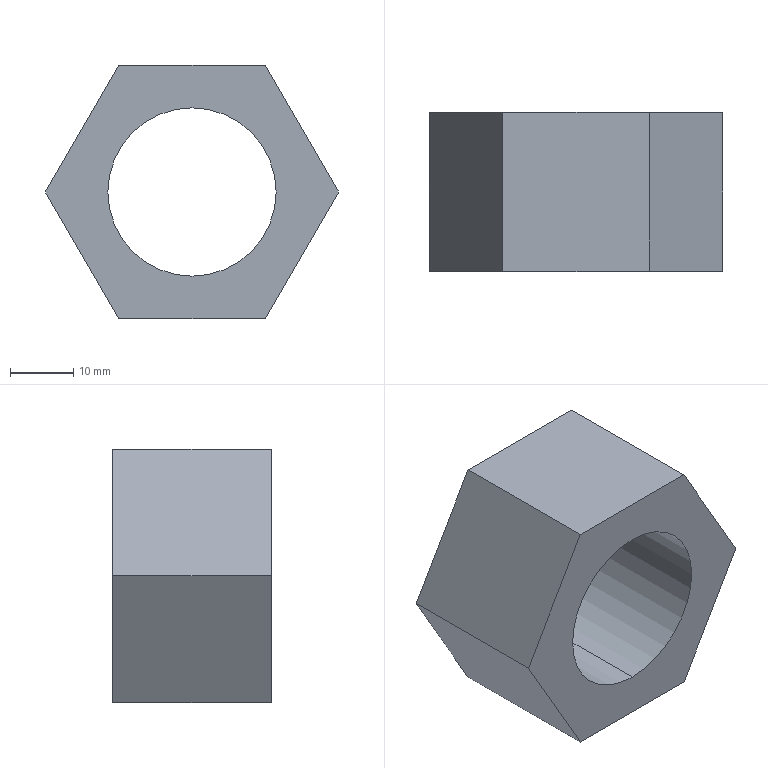Part | STEP file | 1 solid | 10 faces | box 46.188 x 25 x 40 mm | volume 20852 mm3 | plane 8 | cylinder 2 | commonest cylinder face diameters 26.5 x2
STEP:
#1=CARTESIAN_POINT('',(0.,0.,0.));
#2=DIRECTION('',(0.,0.,1.));
#3=DIRECTION('',(1.,0.,0.));
#4=AXIS2_PLACEMENT_3D('',#1,#2,#3);
#5=CARTESIAN_POINT('',(0.,0.,13.25));
#6=VERTEX_POINT('',#5);
#7=CARTESIAN_POINT('',(0.,25.,13.25));
#8=VERTEX_POINT('',#7);
#9=CARTESIAN_POINT('',(0.,0.,13.25));
#10=DIRECTION('',(0.,1.,0.));
#11=VECTOR('',#10,1.);
#12=LINE('',#9,#11);
#13=CARTESIAN_POINT('',(0.,0.,0.));
#14=DIRECTION('',(0.,1.,0.));
#15=DIRECTION('',(0.,0.,1.));
#16=AXIS2_PLACEMENT_3D('',#13,#14,#15);
#17=CYLINDRICAL_SURFACE('',#16,13.25);
#18=CARTESIAN_POINT('',(6.283,0.));
#19=DIRECTION('',(0.,1.));
#20=VECTOR('',#19,1.);
#21=LINE('',#18,#20);
#22=(GEOMETRIC_REPRESENTATION_CONTEXT(2)PARAMETRIC_REPRESENTATION_CONTEXT()REPRESENTATION_CONTEXT('',''));
#23=DEFINITIONAL_REPRESENTATION('',(#21),#22);
#24=PCURVE('',#17,#23);
#25=CARTESIAN_POINT('',(0.,0.,0.));
#26=DIRECTION('',(0.,1.,0.));
#27=DIRECTION('',(0.,0.,1.));
#28=AXIS2_PLACEMENT_3D('',#25,#26,#27);
#29=CYLINDRICAL_SURFACE('',#28,13.25);
#30=CARTESIAN_POINT('',(0.,0.));
#31=DIRECTION('',(0.,1.));
#32=VECTOR('',#31,1.);
#33=LINE('',#30,#32);
#34=(GEOMETRIC_REPRESENTATION_CONTEXT(2)PARAMETRIC_REPRESENTATION_CONTEXT()REPRESENTATION_CONTEXT('',''));
#35=DEFINITIONAL_REPRESENTATION('',(#33),#34);
#36=PCURVE('',#29,#35);
#37=SURFACE_CURVE('',#12,(#24,#36),.PCURVE_S1.);
#38=EDGE_CURVE('',#6,#8,#37,.T.);
#39=ORIENTED_EDGE('',*,*,#38,.T.);
#40=CARTESIAN_POINT('',(0.,25.,-13.25));
#41=VERTEX_POINT('',#40);
#42=CARTESIAN_POINT('',(0.,25.,0.));
#43=DIRECTION('',(0.,1.,0.));
#44=DIRECTION('',(0.,0.,1.));
#45=AXIS2_PLACEMENT_3D('',#42,#43,#44);
#46=CIRCLE('',#45,13.25);
#47=CARTESIAN_POINT('',(0.,25.));
#48=DIRECTION('',(1.,0.));
#49=VECTOR('',#48,1.);
#50=LINE('',#47,#49);
#51=(GEOMETRIC_REPRESENTATION_CONTEXT(2)PARAMETRIC_REPRESENTATION_CONTEXT()REPRESENTATION_CONTEXT('',''));
#52=DEFINITIONAL_REPRESENTATION('',(#50),#51);
#53=PCURVE('',#17,#52);
#54=CARTESIAN_POINT('',(0.,25.,0.));
#55=DIRECTION('',(0.,1.,0.));
#56=DIRECTION('',(0.,0.,1.));
#57=AXIS2_PLACEMENT_3D('',#54,#55,#56);
#58=PLANE('',#57);
#59=CARTESIAN_POINT('',(0.,0.));
#60=DIRECTION('',(1.,0.));
#61=AXIS2_PLACEMENT_2D('',#59,#60);
#62=CIRCLE('',#61,13.25);
#63=(GEOMETRIC_REPRESENTATION_CONTEXT(2)PARAMETRIC_REPRESENTATION_CONTEXT()REPRESENTATION_CONTEXT('',''));
#64=DEFINITIONAL_REPRESENTATION('',(#62),#63);
#65=PCURVE('',#58,#64);
#66=SURFACE_CURVE('',#46,(#53,#65),.PCURVE_S1.);
#67=EDGE_CURVE('',#41,#8,#66,.T.);
#68=ORIENTED_EDGE('',*,*,#67,.F.);
#69=CARTESIAN_POINT('',(0.,0.,-13.25));
#70=VERTEX_POINT('',#69);
#71=CARTESIAN_POINT('',(0.,0.,-13.25));
#72=DIRECTION('',(0.,1.,0.));
#73=VECTOR('',#72,1.);
#74=LINE('',#71,#73);
#75=CARTESIAN_POINT('',(3.142,0.));
#76=DIRECTION('',(0.,1.));
#77=VECTOR('',#76,1.);
#78=LINE('',#75,#77);
#79=(GEOMETRIC_REPRESENTATION_CONTEXT(2)PARAMETRIC_REPRESENTATION_CONTEXT()REPRESENTATION_CONTEXT('',''));
#80=DEFINITIONAL_REPRESENTATION('',(#78),#79);
#81=PCURVE('',#17,#80);
#82=CARTESIAN_POINT('',(3.142,0.));
#83=DIRECTION('',(0.,1.));
#84=VECTOR('',#83,1.);
#85=LINE('',#82,#84);
#86=(GEOMETRIC_REPRESENTATION_CONTEXT(2)PARAMETRIC_REPRESENTATION_CONTEXT()REPRESENTATION_CONTEXT('',''));
#87=DEFINITIONAL_REPRESENTATION('',(#85),#86);
#88=PCURVE('',#29,#87);
#89=SURFACE_CURVE('',#74,(#81,#88),.PCURVE_S1.);
#90=EDGE_CURVE('',#70,#41,#89,.T.);
#91=ORIENTED_EDGE('',*,*,#90,.F.);
#92=CARTESIAN_POINT('',(0.,0.,0.));
#93=DIRECTION('',(0.,1.,0.));
#94=DIRECTION('',(0.,0.,1.));
#95=AXIS2_PLACEMENT_3D('',#92,#93,#94);
#96=CIRCLE('',#95,13.25);
#97=CARTESIAN_POINT('',(0.,0.));
#98=DIRECTION('',(1.,0.));
#99=VECTOR('',#98,1.);
#100=LINE('',#97,#99);
#101=(GEOMETRIC_REPRESENTATION_CONTEXT(2)PARAMETRIC_REPRESENTATION_CONTEXT()REPRESENTATION_CONTEXT('',''));
#102=DEFINITIONAL_REPRESENTATION('',(#100),#101);
#103=PCURVE('',#17,#102);
#104=CARTESIAN_POINT('',(0.,0.,0.));
#105=DIRECTION('',(0.,1.,0.));
#106=DIRECTION('',(0.,0.,1.));
#107=AXIS2_PLACEMENT_3D('',#104,#105,#106);
#108=PLANE('',#107);
#109=CARTESIAN_POINT('',(0.,0.));
#110=DIRECTION('',(1.,0.));
#111=AXIS2_PLACEMENT_2D('',#109,#110);
#112=CIRCLE('',#111,13.25);
#113=(GEOMETRIC_REPRESENTATION_CONTEXT(2)PARAMETRIC_REPRESENTATION_CONTEXT()REPRESENTATION_CONTEXT('',''));
#114=DEFINITIONAL_REPRESENTATION('',(#112),#113);
#115=PCURVE('',#108,#114);
#116=SURFACE_CURVE('',#96,(#103,#115),.PCURVE_S1.);
#117=EDGE_CURVE('',#70,#6,#116,.T.);
#118=ORIENTED_EDGE('',*,*,#117,.T.);
#119=EDGE_LOOP('',(#39,#68,#91,#118));
#120=FACE_BOUND('',#119,.F.);
#121=ADVANCED_FACE('',(#120),#17,.F.);
#122=CARTESIAN_POINT('',(11.547,0.,20.));
#123=VERTEX_POINT('',#122);
#124=CARTESIAN_POINT('',(23.094,0.,0.));
#125=VERTEX_POINT('',#124);
#126=CARTESIAN_POINT('',(11.547,0.,20.));
#127=DIRECTION('',(0.5,0.,-0.866));
#128=VECTOR('',#127,1.);
#129=LINE('',#126,#128);
#130=CARTESIAN_POINT('',(11.547,25.,20.));
#131=DIRECTION('',(-0.866,0.,-0.5));
#132=DIRECTION('',(-0.5,0.,0.866));
#133=AXIS2_PLACEMENT_3D('',#130,#131,#132);
#134=PLANE('',#133);
#135=CARTESIAN_POINT('',(0.,-25.));
#136=DIRECTION('',(-1.,0.));
#137=VECTOR('',#136,1.);
#138=LINE('',#135,#137);
#139=(GEOMETRIC_REPRESENTATION_CONTEXT(2)PARAMETRIC_REPRESENTATION_CONTEXT()REPRESENTATION_CONTEXT('',''));
#140=DEFINITIONAL_REPRESENTATION('',(#138),#139);
#141=PCURVE('',#134,#140);
#142=CARTESIAN_POINT('',(20.,11.547));
#143=DIRECTION('',(-0.866,0.5));
#144=VECTOR('',#143,1.);
#145=LINE('',#142,#144);
#146=(GEOMETRIC_REPRESENTATION_CONTEXT(2)PARAMETRIC_REPRESENTATION_CONTEXT()REPRESENTATION_CONTEXT('',''));
#147=DEFINITIONAL_REPRESENTATION('',(#145),#146);
#148=PCURVE('',#108,#147);
#149=SURFACE_CURVE('',#129,(#141,#148),.PCURVE_S1.);
#150=EDGE_CURVE('',#123,#125,#149,.T.);
#151=ORIENTED_EDGE('',*,*,#150,.T.);
#152=CARTESIAN_POINT('',(23.094,25.,0.));
#153=VERTEX_POINT('',#152);
#154=CARTESIAN_POINT('',(23.094,25.,0.));
#155=DIRECTION('',(0.,-1.,0.));
#156=VECTOR('',#155,1.);
#157=LINE('',#154,#156);
#158=CARTESIAN_POINT('',(-23.094,0.));
#159=DIRECTION('',(0.,-1.));
#160=VECTOR('',#159,1.);
#161=LINE('',#158,#160);
#162=(GEOMETRIC_REPRESENTATION_CONTEXT(2)PARAMETRIC_REPRESENTATION_CONTEXT()REPRESENTATION_CONTEXT('',''));
#163=DEFINITIONAL_REPRESENTATION('',(#161),#162);
#164=PCURVE('',#134,#163);
#165=CARTESIAN_POINT('',(23.094,25.,0.));
#166=DIRECTION('',(-0.866,0.,0.5));
#167=DIRECTION('',(0.5,0.,0.866));
#168=AXIS2_PLACEMENT_3D('',#165,#166,#167);
#169=PLANE('',#168);
#170=CARTESIAN_POINT('',(0.,0.));
#171=DIRECTION('',(0.,-1.));
#172=VECTOR('',#171,1.);
#173=LINE('',#170,#172);
#174=(GEOMETRIC_REPRESENTATION_CONTEXT(2)PARAMETRIC_REPRESENTATION_CONTEXT()REPRESENTATION_CONTEXT('',''));
#175=DEFINITIONAL_REPRESENTATION('',(#173),#174);
#176=PCURVE('',#169,#175);
#177=SURFACE_CURVE('',#157,(#164,#176),.PCURVE_S1.);
#178=EDGE_CURVE('',#153,#125,#177,.T.);
#179=ORIENTED_EDGE('',*,*,#178,.F.);
#180=CARTESIAN_POINT('',(11.547,25.,20.));
#181=VERTEX_POINT('',#180);
#182=CARTESIAN_POINT('',(11.547,25.,20.));
#183=DIRECTION('',(0.5,0.,-0.866));
#184=VECTOR('',#183,1.);
#185=LINE('',#182,#184);
#186=CARTESIAN_POINT('',(0.,0.));
#187=DIRECTION('',(-1.,0.));
#188=VECTOR('',#187,1.);
#189=LINE('',#186,#188);
#190=(GEOMETRIC_REPRESENTATION_CONTEXT(2)PARAMETRIC_REPRESENTATION_CONTEXT()REPRESENTATION_CONTEXT('',''));
#191=DEFINITIONAL_REPRESENTATION('',(#189),#190);
#192=PCURVE('',#134,#191);
#193=CARTESIAN_POINT('',(20.,11.547));
#194=DIRECTION('',(-0.866,0.5));
#195=VECTOR('',#194,1.);
#196=LINE('',#193,#195);
#197=(GEOMETRIC_REPRESENTATION_CONTEXT(2)PARAMETRIC_REPRESENTATION_CONTEXT()REPRESENTATION_CONTEXT('',''));
#198=DEFINITIONAL_REPRESENTATION('',(#196),#197);
#199=PCURVE('',#58,#198);
#200=SURFACE_CURVE('',#185,(#192,#199),.PCURVE_S1.);
#201=EDGE_CURVE('',#181,#153,#200,.T.);
#202=ORIENTED_EDGE('',*,*,#201,.F.);
#203=CARTESIAN_POINT('',(11.547,25.,20.));
#204=DIRECTION('',(0.,-1.,0.));
#205=VECTOR('',#204,1.);
#206=LINE('',#203,#205);
#207=CARTESIAN_POINT('',(0.,0.));
#208=DIRECTION('',(0.,-1.));
#209=VECTOR('',#208,1.);
#210=LINE('',#207,#209);
#211=(GEOMETRIC_REPRESENTATION_CONTEXT(2)PARAMETRIC_REPRESENTATION_CONTEXT()REPRESENTATION_CONTEXT('',''));
#212=DEFINITIONAL_REPRESENTATION('',(#210),#211);
#213=PCURVE('',#134,#212);
#214=CARTESIAN_POINT('',(-11.547,25.,20.));
#215=DIRECTION('',(0.,0.,-1.));
#216=DIRECTION('',(-1.,0.,0.));
#217=AXIS2_PLACEMENT_3D('',#214,#215,#216);
#218=PLANE('',#217);
#219=CARTESIAN_POINT('',(-23.094,0.));
#220=DIRECTION('',(0.,-1.));
#221=VECTOR('',#220,1.);
#222=LINE('',#219,#221);
#223=(GEOMETRIC_REPRESENTATION_CONTEXT(2)PARAMETRIC_REPRESENTATION_CONTEXT()REPRESENTATION_CONTEXT('',''));
#224=DEFINITIONAL_REPRESENTATION('',(#222),#223);
#225=PCURVE('',#218,#224);
#226=SURFACE_CURVE('',#206,(#213,#225),.PCURVE_S1.);
#227=EDGE_CURVE('',#181,#123,#226,.T.);
#228=ORIENTED_EDGE('',*,*,#227,.T.);
#229=EDGE_LOOP('',(#151,#179,#202,#228));
#230=FACE_BOUND('',#229,.T.);
#231=ADVANCED_FACE('',(#230),#134,.F.);
#232=CARTESIAN_POINT('',(11.547,0.,-20.));
#233=VERTEX_POINT('',#232);
#234=CARTESIAN_POINT('',(23.094,0.,0.));
#235=DIRECTION('',(-0.5,0.,-0.866));
#236=VECTOR('',#235,1.);
#237=LINE('',#234,#236);
#238=CARTESIAN_POINT('',(0.,-25.));
#239=DIRECTION('',(-1.,0.));
#240=VECTOR('',#239,1.);
#241=LINE('',#238,#240);
#242=(GEOMETRIC_REPRESENTATION_CONTEXT(2)PARAMETRIC_REPRESENTATION_CONTEXT()REPRESENTATION_CONTEXT('',''));
#243=DEFINITIONAL_REPRESENTATION('',(#241),#242);
#244=PCURVE('',#169,#243);
#245=CARTESIAN_POINT('',(0.,23.094));
#246=DIRECTION('',(-0.866,-0.5));
#247=VECTOR('',#246,1.);
#248=LINE('',#245,#247);
#249=(GEOMETRIC_REPRESENTATION_CONTEXT(2)PARAMETRIC_REPRESENTATION_CONTEXT()REPRESENTATION_CONTEXT('',''));
#250=DEFINITIONAL_REPRESENTATION('',(#248),#249);
#251=PCURVE('',#108,#250);
#252=SURFACE_CURVE('',#237,(#244,#251),.PCURVE_S1.);
#253=EDGE_CURVE('',#125,#233,#252,.T.);
#254=ORIENTED_EDGE('',*,*,#253,.T.);
#255=CARTESIAN_POINT('',(11.547,25.,-20.));
#256=VERTEX_POINT('',#255);
#257=CARTESIAN_POINT('',(11.547,25.,-20.));
#258=DIRECTION('',(0.,-1.,0.));
#259=VECTOR('',#258,1.);
#260=LINE('',#257,#259);
#261=CARTESIAN_POINT('',(-23.094,0.));
#262=DIRECTION('',(0.,-1.));
#263=VECTOR('',#262,1.);
#264=LINE('',#261,#263);
#265=(GEOMETRIC_REPRESENTATION_CONTEXT(2)PARAMETRIC_REPRESENTATION_CONTEXT()REPRESENTATION_CONTEXT('',''));
#266=DEFINITIONAL_REPRESENTATION('',(#264),#265);
#267=PCURVE('',#169,#266);
#268=CARTESIAN_POINT('',(11.547,25.,-20.));
#269=DIRECTION('',(0.,0.,1.));
#270=DIRECTION('',(1.,0.,0.));
#271=AXIS2_PLACEMENT_3D('',#268,#269,#270);
#272=PLANE('',#271);
#273=CARTESIAN_POINT('',(0.,0.));
#274=DIRECTION('',(0.,-1.));
#275=VECTOR('',#274,1.);
#276=LINE('',#273,#275);
#277=(GEOMETRIC_REPRESENTATION_CONTEXT(2)PARAMETRIC_REPRESENTATION_CONTEXT()REPRESENTATION_CONTEXT('',''));
#278=DEFINITIONAL_REPRESENTATION('',(#276),#277);
#279=PCURVE('',#272,#278);
#280=SURFACE_CURVE('',#260,(#267,#279),.PCURVE_S1.);
#281=EDGE_CURVE('',#256,#233,#280,.T.);
#282=ORIENTED_EDGE('',*,*,#281,.F.);
#283=CARTESIAN_POINT('',(23.094,25.,0.));
#284=DIRECTION('',(-0.5,0.,-0.866));
#285=VECTOR('',#284,1.);
#286=LINE('',#283,#285);
#287=CARTESIAN_POINT('',(0.,0.));
#288=DIRECTION('',(-1.,0.));
#289=VECTOR('',#288,1.);
#290=LINE('',#287,#289);
#291=(GEOMETRIC_REPRESENTATION_CONTEXT(2)PARAMETRIC_REPRESENTATION_CONTEXT()REPRESENTATION_CONTEXT('',''));
#292=DEFINITIONAL_REPRESENTATION('',(#290),#291);
#293=PCURVE('',#169,#292);
#294=CARTESIAN_POINT('',(0.,23.094));
#295=DIRECTION('',(-0.866,-0.5));
#296=VECTOR('',#295,1.);
#297=LINE('',#294,#296);
#298=(GEOMETRIC_REPRESENTATION_CONTEXT(2)PARAMETRIC_REPRESENTATION_CONTEXT()REPRESENTATION_CONTEXT('',''));
#299=DEFINITIONAL_REPRESENTATION('',(#297),#298);
#300=PCURVE('',#58,#299);
#301=SURFACE_CURVE('',#286,(#293,#300),.PCURVE_S1.);
#302=EDGE_CURVE('',#153,#256,#301,.T.);
#303=ORIENTED_EDGE('',*,*,#302,.F.);
#304=ORIENTED_EDGE('',*,*,#178,.T.);
#305=EDGE_LOOP('',(#254,#282,#303,#304));
#306=FACE_BOUND('',#305,.T.);
#307=ADVANCED_FACE('',(#306),#169,.F.);
#308=CARTESIAN_POINT('',(-11.547,0.,-20.));
#309=VERTEX_POINT('',#308);
#310=CARTESIAN_POINT('',(11.547,0.,-20.));
#311=DIRECTION('',(-1.,0.,0.));
#312=VECTOR('',#311,1.);
#313=LINE('',#310,#312);
#314=CARTESIAN_POINT('',(0.,-25.));
#315=DIRECTION('',(-1.,0.));
#316=VECTOR('',#315,1.);
#317=LINE('',#314,#316);
#318=(GEOMETRIC_REPRESENTATION_CONTEXT(2)PARAMETRIC_REPRESENTATION_CONTEXT()REPRESENTATION_CONTEXT('',''));
#319=DEFINITIONAL_REPRESENTATION('',(#317),#318);
#320=PCURVE('',#272,#319);
#321=CARTESIAN_POINT('',(-20.,11.547));
#322=DIRECTION('',(0.,-1.));
#323=VECTOR('',#322,1.);
#324=LINE('',#321,#323);
#325=(GEOMETRIC_REPRESENTATION_CONTEXT(2)PARAMETRIC_REPRESENTATION_CONTEXT()REPRESENTATION_CONTEXT('',''));
#326=DEFINITIONAL_REPRESENTATION('',(#324),#325);
#327=PCURVE('',#108,#326);
#328=SURFACE_CURVE('',#313,(#320,#327),.PCURVE_S1.);
#329=EDGE_CURVE('',#233,#309,#328,.T.);
#330=ORIENTED_EDGE('',*,*,#329,.T.);
#331=CARTESIAN_POINT('',(-11.547,25.,-20.));
#332=VERTEX_POINT('',#331);
#333=CARTESIAN_POINT('',(-11.547,25.,-20.));
#334=DIRECTION('',(0.,-1.,0.));
#335=VECTOR('',#334,1.);
#336=LINE('',#333,#335);
#337=CARTESIAN_POINT('',(-23.094,0.));
#338=DIRECTION('',(0.,-1.));
#339=VECTOR('',#338,1.);
#340=LINE('',#337,#339);
#341=(GEOMETRIC_REPRESENTATION_CONTEXT(2)PARAMETRIC_REPRESENTATION_CONTEXT()REPRESENTATION_CONTEXT('',''));
#342=DEFINITIONAL_REPRESENTATION('',(#340),#341);
#343=PCURVE('',#272,#342);
#344=CARTESIAN_POINT('',(-11.547,25.,-20.));
#345=DIRECTION('',(0.866,0.,0.5));
#346=DIRECTION('',(0.5,0.,-0.866));
#347=AXIS2_PLACEMENT_3D('',#344,#345,#346);
#348=PLANE('',#347);
#349=CARTESIAN_POINT('',(0.,0.));
#350=DIRECTION('',(0.,-1.));
#351=VECTOR('',#350,1.);
#352=LINE('',#349,#351);
#353=(GEOMETRIC_REPRESENTATION_CONTEXT(2)PARAMETRIC_REPRESENTATION_CONTEXT()REPRESENTATION_CONTEXT('',''));
#354=DEFINITIONAL_REPRESENTATION('',(#352),#353);
#355=PCURVE('',#348,#354);
#356=SURFACE_CURVE('',#336,(#343,#355),.PCURVE_S1.);
#357=EDGE_CURVE('',#332,#309,#356,.T.);
#358=ORIENTED_EDGE('',*,*,#357,.F.);
#359=CARTESIAN_POINT('',(11.547,25.,-20.));
#360=DIRECTION('',(-1.,0.,0.));
#361=VECTOR('',#360,1.);
#362=LINE('',#359,#361);
#363=CARTESIAN_POINT('',(0.,0.));
#364=DIRECTION('',(-1.,0.));
#365=VECTOR('',#364,1.);
#366=LINE('',#363,#365);
#367=(GEOMETRIC_REPRESENTATION_CONTEXT(2)PARAMETRIC_REPRESENTATION_CONTEXT()REPRESENTATION_CONTEXT('',''));
#368=DEFINITIONAL_REPRESENTATION('',(#366),#367);
#369=PCURVE('',#272,#368);
#370=CARTESIAN_POINT('',(-20.,11.547));
#371=DIRECTION('',(0.,-1.));
#372=VECTOR('',#371,1.);
#373=LINE('',#370,#372);
#374=(GEOMETRIC_REPRESENTATION_CONTEXT(2)PARAMETRIC_REPRESENTATION_CONTEXT()REPRESENTATION_CONTEXT('',''));
#375=DEFINITIONAL_REPRESENTATION('',(#373),#374);
#376=PCURVE('',#58,#375);
#377=SURFACE_CURVE('',#362,(#369,#376),.PCURVE_S1.);
#378=EDGE_CURVE('',#256,#332,#377,.T.);
#379=ORIENTED_EDGE('',*,*,#378,.F.);
#380=ORIENTED_EDGE('',*,*,#281,.T.);
#381=EDGE_LOOP('',(#330,#358,#379,#380));
#382=FACE_BOUND('',#381,.T.);
#383=ADVANCED_FACE('',(#382),#272,.F.);
#384=CARTESIAN_POINT('',(-23.094,0.,0.));
#385=VERTEX_POINT('',#384);
#386=CARTESIAN_POINT('',(-11.547,0.,-20.));
#387=DIRECTION('',(-0.5,0.,0.866));
#388=VECTOR('',#387,1.);
#389=LINE('',#386,#388);
#390=CARTESIAN_POINT('',(0.,-25.));
#391=DIRECTION('',(-1.,0.));
#392=VECTOR('',#391,1.);
#393=LINE('',#390,#392);
#394=(GEOMETRIC_REPRESENTATION_CONTEXT(2)PARAMETRIC_REPRESENTATION_CONTEXT()REPRESENTATION_CONTEXT('',''));
#395=DEFINITIONAL_REPRESENTATION('',(#393),#394);
#396=PCURVE('',#348,#395);
#397=CARTESIAN_POINT('',(-20.,-11.547));
#398=DIRECTION('',(0.866,-0.5));
#399=VECTOR('',#398,1.);
#400=LINE('',#397,#399);
#401=(GEOMETRIC_REPRESENTATION_CONTEXT(2)PARAMETRIC_REPRESENTATION_CONTEXT()REPRESENTATION_CONTEXT('',''));
#402=DEFINITIONAL_REPRESENTATION('',(#400),#401);
#403=PCURVE('',#108,#402);
#404=SURFACE_CURVE('',#389,(#396,#403),.PCURVE_S1.);
#405=EDGE_CURVE('',#309,#385,#404,.T.);
#406=ORIENTED_EDGE('',*,*,#405,.T.);
#407=CARTESIAN_POINT('',(-23.094,25.,0.));
#408=VERTEX_POINT('',#407);
#409=CARTESIAN_POINT('',(-23.094,25.,0.));
#410=DIRECTION('',(0.,-1.,0.));
#411=VECTOR('',#410,1.);
#412=LINE('',#409,#411);
#413=CARTESIAN_POINT('',(-23.094,0.));
#414=DIRECTION('',(0.,-1.));
#415=VECTOR('',#414,1.);
#416=LINE('',#413,#415);
#417=(GEOMETRIC_REPRESENTATION_CONTEXT(2)PARAMETRIC_REPRESENTATION_CONTEXT()REPRESENTATION_CONTEXT('',''));
#418=DEFINITIONAL_REPRESENTATION('',(#416),#417);
#419=PCURVE('',#348,#418);
#420=CARTESIAN_POINT('',(-23.094,25.,0.));
#421=DIRECTION('',(0.866,0.,-0.5));
#422=DIRECTION('',(-0.5,0.,-0.866));
#423=AXIS2_PLACEMENT_3D('',#420,#421,#422);
#424=PLANE('',#423);
#425=CARTESIAN_POINT('',(0.,0.));
#426=DIRECTION('',(0.,-1.));
#427=VECTOR('',#426,1.);
#428=LINE('',#425,#427);
#429=(GEOMETRIC_REPRESENTATION_CONTEXT(2)PARAMETRIC_REPRESENTATION_CONTEXT()REPRESENTATION_CONTEXT('',''));
#430=DEFINITIONAL_REPRESENTATION('',(#428),#429);
#431=PCURVE('',#424,#430);
#432=SURFACE_CURVE('',#412,(#419,#431),.PCURVE_S1.);
#433=EDGE_CURVE('',#408,#385,#432,.T.);
#434=ORIENTED_EDGE('',*,*,#433,.F.);
#435=CARTESIAN_POINT('',(-11.547,25.,-20.));
#436=DIRECTION('',(-0.5,0.,0.866));
#437=VECTOR('',#436,1.);
#438=LINE('',#435,#437);
#439=CARTESIAN_POINT('',(0.,0.));
#440=DIRECTION('',(-1.,0.));
#441=VECTOR('',#440,1.);
#442=LINE('',#439,#441);
#443=(GEOMETRIC_REPRESENTATION_CONTEXT(2)PARAMETRIC_REPRESENTATION_CONTEXT()REPRESENTATION_CONTEXT('',''));
#444=DEFINITIONAL_REPRESENTATION('',(#442),#443);
#445=PCURVE('',#348,#444);
#446=CARTESIAN_POINT('',(-20.,-11.547));
#447=DIRECTION('',(0.866,-0.5));
#448=VECTOR('',#447,1.);
#449=LINE('',#446,#448);
#450=(GEOMETRIC_REPRESENTATION_CONTEXT(2)PARAMETRIC_REPRESENTATION_CONTEXT()REPRESENTATION_CONTEXT('',''));
#451=DEFINITIONAL_REPRESENTATION('',(#449),#450);
#452=PCURVE('',#58,#451);
#453=SURFACE_CURVE('',#438,(#445,#452),.PCURVE_S1.);
#454=EDGE_CURVE('',#332,#408,#453,.T.);
#455=ORIENTED_EDGE('',*,*,#454,.F.);
#456=ORIENTED_EDGE('',*,*,#357,.T.);
#457=EDGE_LOOP('',(#406,#434,#455,#456));
#458=FACE_BOUND('',#457,.T.);
#459=ADVANCED_FACE('',(#458),#348,.F.);
#460=CARTESIAN_POINT('',(-11.547,0.,20.));
#461=VERTEX_POINT('',#460);
#462=CARTESIAN_POINT('',(-23.094,0.,0.));
#463=DIRECTION('',(0.5,0.,0.866));
#464=VECTOR('',#463,1.);
#465=LINE('',#462,#464);
#466=CARTESIAN_POINT('',(0.,-25.));
#467=DIRECTION('',(-1.,0.));
#468=VECTOR('',#467,1.);
#469=LINE('',#466,#468);
#470=(GEOMETRIC_REPRESENTATION_CONTEXT(2)PARAMETRIC_REPRESENTATION_CONTEXT()REPRESENTATION_CONTEXT('',''));
#471=DEFINITIONAL_REPRESENTATION('',(#469),#470);
#472=PCURVE('',#424,#471);
#473=CARTESIAN_POINT('',(0.,-23.094));
#474=DIRECTION('',(0.866,0.5));
#475=VECTOR('',#474,1.);
#476=LINE('',#473,#475);
#477=(GEOMETRIC_REPRESENTATION_CONTEXT(2)PARAMETRIC_REPRESENTATION_CONTEXT()REPRESENTATION_CONTEXT('',''));
#478=DEFINITIONAL_REPRESENTATION('',(#476),#477);
#479=PCURVE('',#108,#478);
#480=SURFACE_CURVE('',#465,(#472,#479),.PCURVE_S1.);
#481=EDGE_CURVE('',#385,#461,#480,.T.);
#482=ORIENTED_EDGE('',*,*,#481,.T.);
#483=CARTESIAN_POINT('',(-11.547,25.,20.));
#484=VERTEX_POINT('',#483);
#485=CARTESIAN_POINT('',(-11.547,25.,20.));
#486=DIRECTION('',(0.,-1.,0.));
#487=VECTOR('',#486,1.);
#488=LINE('',#485,#487);
#489=CARTESIAN_POINT('',(-23.094,0.));
#490=DIRECTION('',(0.,-1.));
#491=VECTOR('',#490,1.);
#492=LINE('',#489,#491);
#493=(GEOMETRIC_REPRESENTATION_CONTEXT(2)PARAMETRIC_REPRESENTATION_CONTEXT()REPRESENTATION_CONTEXT('',''));
#494=DEFINITIONAL_REPRESENTATION('',(#492),#493);
#495=PCURVE('',#424,#494);
#496=CARTESIAN_POINT('',(0.,0.));
#497=DIRECTION('',(0.,-1.));
#498=VECTOR('',#497,1.);
#499=LINE('',#496,#498);
#500=(GEOMETRIC_REPRESENTATION_CONTEXT(2)PARAMETRIC_REPRESENTATION_CONTEXT()REPRESENTATION_CONTEXT('',''));
#501=DEFINITIONAL_REPRESENTATION('',(#499),#500);
#502=PCURVE('',#218,#501);
#503=SURFACE_CURVE('',#488,(#495,#502),.PCURVE_S1.);
#504=EDGE_CURVE('',#484,#461,#503,.T.);
#505=ORIENTED_EDGE('',*,*,#504,.F.);
#506=CARTESIAN_POINT('',(-23.094,25.,0.));
#507=DIRECTION('',(0.5,0.,0.866));
#508=VECTOR('',#507,1.);
#509=LINE('',#506,#508);
#510=CARTESIAN_POINT('',(0.,0.));
#511=DIRECTION('',(-1.,0.));
#512=VECTOR('',#511,1.);
#513=LINE('',#510,#512);
#514=(GEOMETRIC_REPRESENTATION_CONTEXT(2)PARAMETRIC_REPRESENTATION_CONTEXT()REPRESENTATION_CONTEXT('',''));
#515=DEFINITIONAL_REPRESENTATION('',(#513),#514);
#516=PCURVE('',#424,#515);
#517=CARTESIAN_POINT('',(0.,-23.094));
#518=DIRECTION('',(0.866,0.5));
#519=VECTOR('',#518,1.);
#520=LINE('',#517,#519);
#521=(GEOMETRIC_REPRESENTATION_CONTEXT(2)PARAMETRIC_REPRESENTATION_CONTEXT()REPRESENTATION_CONTEXT('',''));
#522=DEFINITIONAL_REPRESENTATION('',(#520),#521);
#523=PCURVE('',#58,#522);
#524=SURFACE_CURVE('',#509,(#516,#523),.PCURVE_S1.);
#525=EDGE_CURVE('',#408,#484,#524,.T.);
#526=ORIENTED_EDGE('',*,*,#525,.F.);
#527=ORIENTED_EDGE('',*,*,#433,.T.);
#528=EDGE_LOOP('',(#482,#505,#526,#527));
#529=FACE_BOUND('',#528,.T.);
#530=ADVANCED_FACE('',(#529),#424,.F.);
#531=CARTESIAN_POINT('',(-11.547,0.,20.));
#532=DIRECTION('',(1.,0.,0.));
#533=VECTOR('',#532,1.);
#534=LINE('',#531,#533);
#535=CARTESIAN_POINT('',(0.,-25.));
#536=DIRECTION('',(-1.,0.));
#537=VECTOR('',#536,1.);
#538=LINE('',#535,#537);
#539=(GEOMETRIC_REPRESENTATION_CONTEXT(2)PARAMETRIC_REPRESENTATION_CONTEXT()REPRESENTATION_CONTEXT('',''));
#540=DEFINITIONAL_REPRESENTATION('',(#538),#539);
#541=PCURVE('',#218,#540);
#542=CARTESIAN_POINT('',(20.,-11.547));
#543=DIRECTION('',(0.,1.));
#544=VECTOR('',#543,1.);
#545=LINE('',#542,#544);
#546=(GEOMETRIC_REPRESENTATION_CONTEXT(2)PARAMETRIC_REPRESENTATION_CONTEXT()REPRESENTATION_CONTEXT('',''));
#547=DEFINITIONAL_REPRESENTATION('',(#545),#546);
#548=PCURVE('',#108,#547);
#549=SURFACE_CURVE('',#534,(#541,#548),.PCURVE_S1.);
#550=EDGE_CURVE('',#461,#123,#549,.T.);
#551=ORIENTED_EDGE('',*,*,#550,.T.);
#552=ORIENTED_EDGE('',*,*,#227,.F.);
#553=CARTESIAN_POINT('',(-11.547,25.,20.));
#554=DIRECTION('',(1.,0.,0.));
#555=VECTOR('',#554,1.);
#556=LINE('',#553,#555);
#557=CARTESIAN_POINT('',(0.,0.));
#558=DIRECTION('',(-1.,0.));
#559=VECTOR('',#558,1.);
#560=LINE('',#557,#559);
#561=(GEOMETRIC_REPRESENTATION_CONTEXT(2)PARAMETRIC_REPRESENTATION_CONTEXT()REPRESENTATION_CONTEXT('',''));
#562=DEFINITIONAL_REPRESENTATION('',(#560),#561);
#563=PCURVE('',#218,#562);
#564=CARTESIAN_POINT('',(20.,-11.547));
#565=DIRECTION('',(0.,1.));
#566=VECTOR('',#565,1.);
#567=LINE('',#564,#566);
#568=(GEOMETRIC_REPRESENTATION_CONTEXT(2)PARAMETRIC_REPRESENTATION_CONTEXT()REPRESENTATION_CONTEXT('',''));
#569=DEFINITIONAL_REPRESENTATION('',(#567),#568);
#570=PCURVE('',#58,#569);
#571=SURFACE_CURVE('',#556,(#563,#570),.PCURVE_S1.);
#572=EDGE_CURVE('',#484,#181,#571,.T.);
#573=ORIENTED_EDGE('',*,*,#572,.F.);
#574=ORIENTED_EDGE('',*,*,#504,.T.);
#575=EDGE_LOOP('',(#551,#552,#573,#574));
#576=FACE_BOUND('',#575,.T.);
#577=ADVANCED_FACE('',(#576),#218,.F.);
#578=CARTESIAN_POINT('',(0.,25.,0.));
#579=DIRECTION('',(0.,1.,0.));
#580=DIRECTION('',(0.,0.,1.));
#581=AXIS2_PLACEMENT_3D('',#578,#579,#580);
#582=CIRCLE('',#581,13.25);
#583=CARTESIAN_POINT('',(0.,0.));
#584=DIRECTION('',(1.,0.));
#585=AXIS2_PLACEMENT_2D('',#583,#584);
#586=CIRCLE('',#585,13.25);
#587=(GEOMETRIC_REPRESENTATION_CONTEXT(2)PARAMETRIC_REPRESENTATION_CONTEXT()REPRESENTATION_CONTEXT('',''));
#588=DEFINITIONAL_REPRESENTATION('',(#586),#587);
#589=PCURVE('',#58,#588);
#590=CARTESIAN_POINT('',(0.,25.));
#591=DIRECTION('',(1.,0.));
#592=VECTOR('',#591,1.);
#593=LINE('',#590,#592);
#594=(GEOMETRIC_REPRESENTATION_CONTEXT(2)PARAMETRIC_REPRESENTATION_CONTEXT()REPRESENTATION_CONTEXT('',''));
#595=DEFINITIONAL_REPRESENTATION('',(#593),#594);
#596=PCURVE('',#29,#595);
#597=SURFACE_CURVE('',#582,(#589,#596),.PCURVE_S1.);
#598=EDGE_CURVE('',#8,#41,#597,.T.);
#599=ORIENTED_EDGE('',*,*,#598,.F.);
#600=ORIENTED_EDGE('',*,*,#67,.F.);
#601=EDGE_LOOP('',(#599,#600));
#602=FACE_BOUND('',#601,.T.);
#603=ORIENTED_EDGE('',*,*,#201,.T.);
#604=ORIENTED_EDGE('',*,*,#302,.T.);
#605=ORIENTED_EDGE('',*,*,#378,.T.);
#606=ORIENTED_EDGE('',*,*,#454,.T.);
#607=ORIENTED_EDGE('',*,*,#525,.T.);
#608=ORIENTED_EDGE('',*,*,#572,.T.);
#609=EDGE_LOOP('',(#603,#604,#605,#606,#607,#608));
#610=FACE_BOUND('',#609,.T.);
#611=ADVANCED_FACE('',(#602,#610),#58,.T.);
#612=CARTESIAN_POINT('',(0.,0.,0.));
#613=DIRECTION('',(0.,1.,0.));
#614=DIRECTION('',(0.,0.,1.));
#615=AXIS2_PLACEMENT_3D('',#612,#613,#614);
#616=CIRCLE('',#615,13.25);
#617=CARTESIAN_POINT('',(0.,0.));
#618=DIRECTION('',(1.,0.));
#619=AXIS2_PLACEMENT_2D('',#617,#618);
#620=CIRCLE('',#619,13.25);
#621=(GEOMETRIC_REPRESENTATION_CONTEXT(2)PARAMETRIC_REPRESENTATION_CONTEXT()REPRESENTATION_CONTEXT('',''));
#622=DEFINITIONAL_REPRESENTATION('',(#620),#621);
#623=PCURVE('',#108,#622);
#624=CARTESIAN_POINT('',(0.,0.));
#625=DIRECTION('',(1.,0.));
#626=VECTOR('',#625,1.);
#627=LINE('',#624,#626);
#628=(GEOMETRIC_REPRESENTATION_CONTEXT(2)PARAMETRIC_REPRESENTATION_CONTEXT()REPRESENTATION_CONTEXT('',''));
#629=DEFINITIONAL_REPRESENTATION('',(#627),#628);
#630=PCURVE('',#29,#629);
#631=SURFACE_CURVE('',#616,(#623,#630),.PCURVE_S1.);
#632=EDGE_CURVE('',#6,#70,#631,.T.);
#633=ORIENTED_EDGE('',*,*,#632,.T.);
#634=ORIENTED_EDGE('',*,*,#117,.T.);
#635=EDGE_LOOP('',(#633,#634));
#636=FACE_BOUND('',#635,.T.);
#637=ORIENTED_EDGE('',*,*,#150,.F.);
#638=ORIENTED_EDGE('',*,*,#550,.F.);
#639=ORIENTED_EDGE('',*,*,#481,.F.);
#640=ORIENTED_EDGE('',*,*,#405,.F.);
#641=ORIENTED_EDGE('',*,*,#329,.F.);
#642=ORIENTED_EDGE('',*,*,#253,.F.);
#643=EDGE_LOOP('',(#637,#638,#639,#640,#641,#642));
#644=FACE_BOUND('',#643,.T.);
#645=ADVANCED_FACE('',(#636,#644),#108,.F.);
#646=ORIENTED_EDGE('',*,*,#598,.F.);
#647=ORIENTED_EDGE('',*,*,#38,.F.);
#648=ORIENTED_EDGE('',*,*,#632,.T.);
#649=ORIENTED_EDGE('',*,*,#90,.T.);
#650=EDGE_LOOP('',(#646,#647,#648,#649));
#651=FACE_BOUND('',#650,.F.);
#652=ADVANCED_FACE('',(#651),#29,.F.);
#653=CLOSED_SHELL('',(#121,#231,#307,#383,#459,#530,#577,#611,#645,#652));
#654=MANIFOLD_SOLID_BREP('',#653);
#655=(LENGTH_UNIT()NAMED_UNIT(*)SI_UNIT(.MILLI.,.METRE.));
#656=UNCERTAINTY_MEASURE_WITH_UNIT(LENGTH_MEASURE(0.0000001),#655,'','');
#657=(NAMED_UNIT(*)PLANE_ANGLE_UNIT()SI_UNIT($,.RADIAN.));
#658=(NAMED_UNIT(*)SI_UNIT($,.STERADIAN.)SOLID_ANGLE_UNIT());
#659=(GEOMETRIC_REPRESENTATION_CONTEXT(3)GLOBAL_UNCERTAINTY_ASSIGNED_CONTEXT((#656))GLOBAL_UNIT_ASSIGNED_CONTEXT((#655,#657,#658))REPRESENTATION_CONTEXT('',''));
#660=ADVANCED_BREP_SHAPE_REPRESENTATION('',(#4,#654),#659);